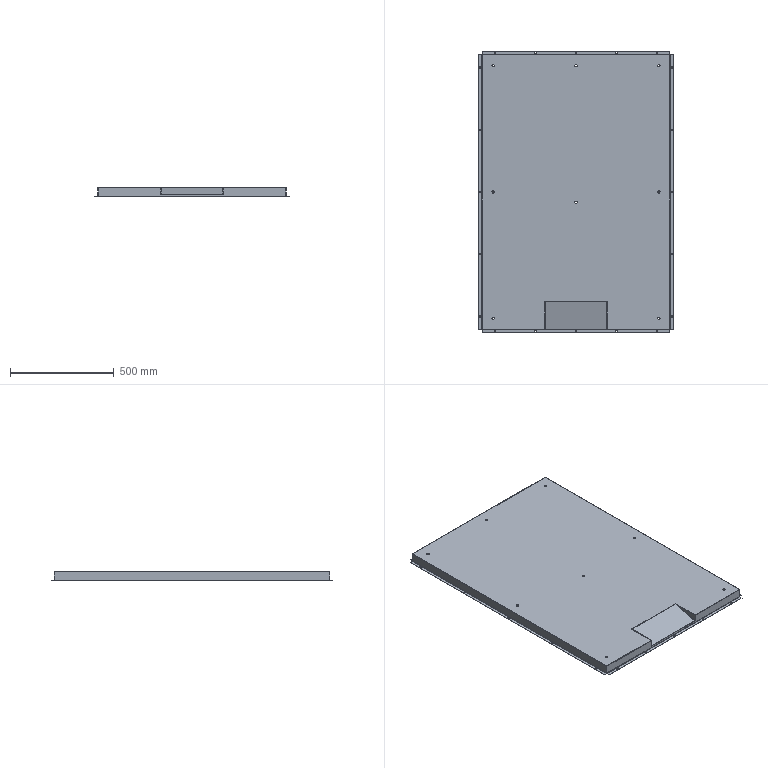Part | SolidWorks | 2 solids | 206 faces | box 940 x 1360 x 44 mm | volume 1458803 mm3 | plane 106 | cylinder 88 | spline 12 | commonest cylinder face diameters 7 x50 11 x16 1 x9 3 x9 0.4 x2 2.4 x2